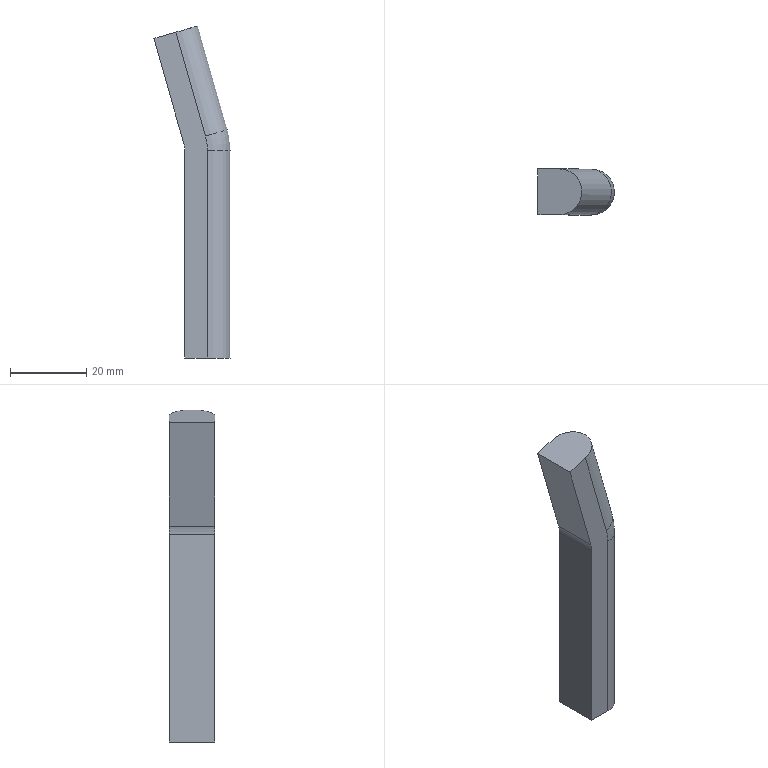Part | NX | features solid 2 | 1 solid | 10 faces | box 20.071 x 12 x 87.272 mm | volume 11133 mm3 | plane 6 | cylinder 3 | torus 1 | commonest cylinder face diameters 12 x2 16 x1
STEP:
#1=CARTESIAN_POINT('',(-548.,484.,14.523));
#2=VERTEX_POINT('',#1);
#3=CARTESIAN_POINT('',(-548.,496.,14.523));
#4=VERTEX_POINT('',#3);
#5=CARTESIAN_POINT('',(-548.,520.,14.523));
#6=DIRECTION('',(0.,1.,0.));
#7=VECTOR('',#6,1000.);
#8=LINE('',#5,#7);
#9=EDGE_CURVE('',#2,#4,#8,.T.);
#10=ORIENTED_EDGE('',*,*,#9,.T.);
#11=CARTESIAN_POINT('',(-548.,496.,-40.));
#12=VERTEX_POINT('',#11);
#13=CARTESIAN_POINT('',(-548.,496.,49.523));
#14=DIRECTION('',(0.,0.,-1.));
#15=VECTOR('',#14,1000.);
#16=LINE('',#13,#15);
#17=EDGE_CURVE('',#4,#12,#16,.T.);
#18=ORIENTED_EDGE('',*,*,#17,.T.);
#19=CARTESIAN_POINT('',(-548.,484.,-40.));
#20=VERTEX_POINT('',#19);
#21=CARTESIAN_POINT('',(-548.,463.,-40.));
#22=DIRECTION('',(0.,1.,0.));
#23=VECTOR('',#22,1000.);
#24=LINE('',#21,#23);
#25=EDGE_CURVE('',#20,#12,#24,.T.);
#26=ORIENTED_EDGE('',*,*,#25,.F.);
#27=CARTESIAN_POINT('',(-548.,484.,49.523));
#28=DIRECTION('',(0.,0.,-1.));
#29=VECTOR('',#28,1000.);
#30=LINE('',#27,#29);
#31=EDGE_CURVE('',#2,#20,#30,.T.);
#32=ORIENTED_EDGE('',*,*,#31,.F.);
#33=EDGE_LOOP('',(#10,#18,#26,#32));
#34=FACE_BOUND('',#33,.T.);
#35=CARTESIAN_POINT('',(-548.,520.,49.523));
#36=DIRECTION('',(1.,0.,0.));
#37=DIRECTION('',(0.,-1.,0.));
#38=AXIS2_PLACEMENT_3D('',#35,#36,#37);
#39=PLANE('',#38);
#40=ADVANCED_FACE('',(#34),#39,.F.);
#41=CARTESIAN_POINT('',(-542.,496.,14.523));
#42=VERTEX_POINT('',#41);
#43=CARTESIAN_POINT('',(-542.,484.,14.523));
#44=VERTEX_POINT('',#43);
#45=CARTESIAN_POINT('',(-542.,490.,14.523));
#46=DIRECTION('',(0.,0.,-1.));
#47=DIRECTION('',(1.,0.,0.));
#48=AXIS2_PLACEMENT_3D('',#45,#46,#47);
#49=CIRCLE('',#48,6.);
#50=EDGE_CURVE('',#42,#44,#49,.T.);
#51=ORIENTED_EDGE('',*,*,#50,.F.);
#52=CARTESIAN_POINT('',(-542.535,496.,18.357));
#53=VERTEX_POINT('',#52);
#54=CARTESIAN_POINT('',(-556.,496.,14.523));
#55=DIRECTION('',(0.,-1.,0.));
#56=DIRECTION('',(0.,0.,-1.));
#57=AXIS2_PLACEMENT_3D('',#54,#55,#56);
#58=CIRCLE('',#57,14.);
#59=EDGE_CURVE('',#42,#53,#58,.T.);
#60=ORIENTED_EDGE('',*,*,#59,.T.);
#61=CARTESIAN_POINT('',(-542.535,484.,18.357));
#62=VERTEX_POINT('',#61);
#63=CARTESIAN_POINT('',(-542.535,490.,18.357));
#64=DIRECTION('',(0.2738,0.,-0.9618));
#65=DIRECTION('',(0.9618,0.,0.2738));
#66=AXIS2_PLACEMENT_3D('',#63,#64,#65);
#67=CIRCLE('',#66,6.);
#68=EDGE_CURVE('',#53,#62,#67,.T.);
#69=ORIENTED_EDGE('',*,*,#68,.T.);
#70=CARTESIAN_POINT('',(-556.,484.,14.523));
#71=DIRECTION('',(0.,-1.,0.));
#72=DIRECTION('',(0.,0.,-1.));
#73=AXIS2_PLACEMENT_3D('',#70,#71,#72);
#74=CIRCLE('',#73,14.);
#75=EDGE_CURVE('',#44,#62,#74,.T.);
#76=ORIENTED_EDGE('',*,*,#75,.F.);
#77=EDGE_LOOP('',(#51,#60,#69,#76));
#78=FACE_BOUND('',#77,.T.);
#79=CARTESIAN_POINT('',(-556.,490.,14.523));
#80=DIRECTION('',(0.,1.,0.));
#81=DIRECTION('',(0.,0.,-1.));
#82=AXIS2_PLACEMENT_3D('',#79,#80,#81);
#83=TOROIDAL_SURFACE('',#82,14.,6.);
#84=ADVANCED_FACE('',(#78),#83,.T.);
#85=ORIENTED_EDGE('',*,*,#50,.T.);
#86=CARTESIAN_POINT('',(-542.,484.,-40.));
#87=VERTEX_POINT('',#86);
#88=CARTESIAN_POINT('',(-542.,484.,29.523));
#89=DIRECTION('',(0.,0.,-1.));
#90=VECTOR('',#89,1000.);
#91=LINE('',#88,#90);
#92=EDGE_CURVE('',#44,#87,#91,.T.);
#93=ORIENTED_EDGE('',*,*,#92,.T.);
#94=CARTESIAN_POINT('',(-542.,496.,-40.));
#95=VERTEX_POINT('',#94);
#96=CARTESIAN_POINT('',(-542.,490.,-40.));
#97=DIRECTION('',(0.,0.,1.));
#98=DIRECTION('',(1.,0.,0.));
#99=AXIS2_PLACEMENT_3D('',#96,#97,#98);
#100=CIRCLE('',#99,6.);
#101=EDGE_CURVE('',#95,#87,#100,.F.);
#102=ORIENTED_EDGE('',*,*,#101,.F.);
#103=CARTESIAN_POINT('',(-542.,496.,29.523));
#104=DIRECTION('',(0.,0.,-1.));
#105=VECTOR('',#104,1000.);
#106=LINE('',#103,#105);
#107=EDGE_CURVE('',#42,#95,#106,.T.);
#108=ORIENTED_EDGE('',*,*,#107,.F.);
#109=EDGE_LOOP('',(#85,#93,#102,#108));
#110=FACE_BOUND('',#109,.T.);
#111=CARTESIAN_POINT('',(-542.,490.,29.523));
#112=DIRECTION('',(0.,0.,-1.));
#113=DIRECTION('',(-1.,0.,0.));
#114=AXIS2_PLACEMENT_3D('',#111,#112,#113);
#115=CYLINDRICAL_SURFACE('',#114,6.);
#116=ADVANCED_FACE('',(#110),#115,.T.);
#117=CARTESIAN_POINT('',(-623.,484.,-40.));
#118=DIRECTION('',(-1.,0.,0.));
#119=VECTOR('',#118,1000.);
#120=LINE('',#117,#119);
#121=EDGE_CURVE('',#87,#20,#120,.T.);
#122=ORIENTED_EDGE('',*,*,#121,.T.);
#123=ORIENTED_EDGE('',*,*,#25,.T.);
#124=CARTESIAN_POINT('',(-623.,496.,-40.));
#125=DIRECTION('',(-1.,0.,0.));
#126=VECTOR('',#125,1000.);
#127=LINE('',#124,#126);
#128=EDGE_CURVE('',#95,#12,#127,.T.);
#129=ORIENTED_EDGE('',*,*,#128,.F.);
#130=ORIENTED_EDGE('',*,*,#101,.T.);
#131=EDGE_LOOP('',(#122,#123,#129,#130));
#132=FACE_BOUND('',#131,.T.);
#133=CARTESIAN_POINT('',(-623.,463.,-40.));
#134=DIRECTION('',(0.,0.,1.));
#135=DIRECTION('',(0.,1.,0.));
#136=AXIS2_PLACEMENT_3D('',#133,#134,#135);
#137=PLANE('',#136);
#138=ADVANCED_FACE('',(#132),#137,.F.);
#139=CARTESIAN_POINT('',(-550.3,484.,45.629));
#140=VERTEX_POINT('',#139);
#141=CARTESIAN_POINT('',(-542.535,484.,18.357));
#142=DIRECTION('',(-0.2738,0.,0.9618));
#143=VECTOR('',#142,1000.);
#144=LINE('',#141,#143);
#145=EDGE_CURVE('',#62,#140,#144,.T.);
#146=ORIENTED_EDGE('',*,*,#145,.T.);
#147=CARTESIAN_POINT('',(-556.071,484.,43.986));
#148=VERTEX_POINT('',#147);
#149=CARTESIAN_POINT('',(-557.81,484.,43.491));
#150=DIRECTION('',(-0.9618,0.,-0.2738));
#151=VECTOR('',#150,1000.);
#152=LINE('',#149,#151);
#153=EDGE_CURVE('',#140,#148,#152,.T.);
#154=ORIENTED_EDGE('',*,*,#153,.T.);
#155=CARTESIAN_POINT('',(-548.306,484.,16.714));
#156=VERTEX_POINT('',#155);
#157=CARTESIAN_POINT('',(-548.306,484.,16.714));
#158=DIRECTION('',(-0.2738,0.,0.9618));
#159=VECTOR('',#158,1000.);
#160=LINE('',#157,#159);
#161=EDGE_CURVE('',#156,#148,#160,.T.);
#162=ORIENTED_EDGE('',*,*,#161,.F.);
#163=CARTESIAN_POINT('',(-556.,484.,14.523));
#164=DIRECTION('',(0.,-1.,0.));
#165=DIRECTION('',(0.,0.,-1.));
#166=AXIS2_PLACEMENT_3D('',#163,#164,#165);
#167=CIRCLE('',#166,8.);
#168=EDGE_CURVE('',#2,#156,#167,.T.);
#169=ORIENTED_EDGE('',*,*,#168,.F.);
#170=ORIENTED_EDGE('',*,*,#31,.T.);
#171=ORIENTED_EDGE('',*,*,#121,.F.);
#172=ORIENTED_EDGE('',*,*,#92,.F.);
#173=ORIENTED_EDGE('',*,*,#75,.T.);
#174=EDGE_LOOP('',(#146,#154,#162,#169,#170,#171,#172,#173));
#175=FACE_BOUND('',#174,.T.);
#176=CARTESIAN_POINT('',(-640.,484.,39.523));
#177=DIRECTION('',(0.,1.,0.));
#178=DIRECTION('',(1.,0.,0.));
#179=AXIS2_PLACEMENT_3D('',#176,#177,#178);
#180=PLANE('',#179);
#181=ADVANCED_FACE('',(#175),#180,.F.);
#182=ORIENTED_EDGE('',*,*,#17,.F.);
#183=CARTESIAN_POINT('',(-548.306,496.,16.714));
#184=VERTEX_POINT('',#183);
#185=CARTESIAN_POINT('',(-556.,496.,14.523));
#186=DIRECTION('',(0.,-1.,0.));
#187=DIRECTION('',(0.,0.,-1.));
#188=AXIS2_PLACEMENT_3D('',#185,#186,#187);
#189=CIRCLE('',#188,8.);
#190=EDGE_CURVE('',#4,#184,#189,.T.);
#191=ORIENTED_EDGE('',*,*,#190,.T.);
#192=CARTESIAN_POINT('',(-556.071,496.,43.986));
#193=VERTEX_POINT('',#192);
#194=CARTESIAN_POINT('',(-548.306,496.,16.714));
#195=DIRECTION('',(-0.2738,0.,0.9618));
#196=VECTOR('',#195,1000.);
#197=LINE('',#194,#196);
#198=EDGE_CURVE('',#184,#193,#197,.T.);
#199=ORIENTED_EDGE('',*,*,#198,.T.);
#200=CARTESIAN_POINT('',(-550.3,496.,45.629));
#201=VERTEX_POINT('',#200);
#202=CARTESIAN_POINT('',(-557.81,496.,43.491));
#203=DIRECTION('',(-0.9618,0.,-0.2738));
#204=VECTOR('',#203,1000.);
#205=LINE('',#202,#204);
#206=EDGE_CURVE('',#201,#193,#205,.T.);
#207=ORIENTED_EDGE('',*,*,#206,.F.);
#208=CARTESIAN_POINT('',(-542.535,496.,18.357));
#209=DIRECTION('',(-0.2738,0.,0.9618));
#210=VECTOR('',#209,1000.);
#211=LINE('',#208,#210);
#212=EDGE_CURVE('',#53,#201,#211,.T.);
#213=ORIENTED_EDGE('',*,*,#212,.F.);
#214=ORIENTED_EDGE('',*,*,#59,.F.);
#215=ORIENTED_EDGE('',*,*,#107,.T.);
#216=ORIENTED_EDGE('',*,*,#128,.T.);
#217=EDGE_LOOP('',(#182,#191,#199,#207,#213,#214,#215,#216));
#218=FACE_BOUND('',#217,.T.);
#219=CARTESIAN_POINT('',(-640.,496.,39.523));
#220=DIRECTION('',(0.,1.,0.));
#221=DIRECTION('',(1.,0.,0.));
#222=AXIS2_PLACEMENT_3D('',#219,#220,#221);
#223=PLANE('',#222);
#224=ADVANCED_FACE('',(#218),#223,.T.);
#225=CARTESIAN_POINT('',(-550.3,490.,45.629));
#226=DIRECTION('',(-0.2738,0.,0.9618));
#227=DIRECTION('',(0.9618,0.,0.2738));
#228=AXIS2_PLACEMENT_3D('',#225,#226,#227);
#229=CIRCLE('',#228,6.);
#230=EDGE_CURVE('',#201,#140,#229,.F.);
#231=ORIENTED_EDGE('',*,*,#230,.F.);
#232=ORIENTED_EDGE('',*,*,#206,.T.);
#233=CARTESIAN_POINT('',(-556.071,520.,43.986));
#234=DIRECTION('',(0.,1.,0.));
#235=VECTOR('',#234,1000.);
#236=LINE('',#233,#235);
#237=EDGE_CURVE('',#148,#193,#236,.T.);
#238=ORIENTED_EDGE('',*,*,#237,.F.);
#239=ORIENTED_EDGE('',*,*,#153,.F.);
#240=EDGE_LOOP('',(#231,#232,#238,#239));
#241=FACE_BOUND('',#240,.T.);
#242=CARTESIAN_POINT('',(-557.81,549.75,43.491));
#243=DIRECTION('',(-0.2738,0.,0.9618));
#244=DIRECTION('',(0.9618,0.,0.2738));
#245=AXIS2_PLACEMENT_3D('',#242,#243,#244);
#246=PLANE('',#245);
#247=ADVANCED_FACE('',(#241),#246,.T.);
#248=ORIENTED_EDGE('',*,*,#212,.T.);
#249=ORIENTED_EDGE('',*,*,#230,.T.);
#250=ORIENTED_EDGE('',*,*,#145,.F.);
#251=ORIENTED_EDGE('',*,*,#68,.F.);
#252=EDGE_LOOP('',(#248,#249,#250,#251));
#253=FACE_BOUND('',#252,.T.);
#254=CARTESIAN_POINT('',(-542.535,490.,18.357));
#255=DIRECTION('',(-0.2738,0.,0.9618));
#256=DIRECTION('',(0.9618,0.,0.2738));
#257=AXIS2_PLACEMENT_3D('',#254,#255,#256);
#258=CYLINDRICAL_SURFACE('',#257,6.);
#259=ADVANCED_FACE('',(#253),#258,.T.);
#260=CARTESIAN_POINT('',(-548.306,520.,16.714));
#261=DIRECTION('',(0.,1.,0.));
#262=VECTOR('',#261,1000.);
#263=LINE('',#260,#262);
#264=EDGE_CURVE('',#156,#184,#263,.T.);
#265=ORIENTED_EDGE('',*,*,#264,.F.);
#266=ORIENTED_EDGE('',*,*,#161,.T.);
#267=ORIENTED_EDGE('',*,*,#237,.T.);
#268=ORIENTED_EDGE('',*,*,#198,.F.);
#269=EDGE_LOOP('',(#265,#266,#267,#268));
#270=FACE_BOUND('',#269,.T.);
#271=CARTESIAN_POINT('',(-548.306,520.,16.714));
#272=DIRECTION('',(-0.9618,0.,-0.2738));
#273=DIRECTION('',(-0.2738,0.,0.9618));
#274=AXIS2_PLACEMENT_3D('',#271,#272,#273);
#275=PLANE('',#274);
#276=ADVANCED_FACE('',(#270),#275,.T.);
#277=ORIENTED_EDGE('',*,*,#9,.F.);
#278=ORIENTED_EDGE('',*,*,#168,.T.);
#279=ORIENTED_EDGE('',*,*,#264,.T.);
#280=ORIENTED_EDGE('',*,*,#190,.F.);
#281=EDGE_LOOP('',(#277,#278,#279,#280));
#282=FACE_BOUND('',#281,.T.);
#283=CARTESIAN_POINT('',(-556.,535.,14.523));
#284=DIRECTION('',(0.,1.,0.));
#285=DIRECTION('',(0.,0.,-1.));
#286=AXIS2_PLACEMENT_3D('',#283,#284,#285);
#287=CYLINDRICAL_SURFACE('',#286,8.);
#288=ADVANCED_FACE('',(#282),#287,.F.);
#289=CLOSED_SHELL('',(#40,#84,#116,#138,#181,#224,#247,#259,#276,#288));
#290=MANIFOLD_SOLID_BREP('',#289);
#291=(LENGTH_UNIT()NAMED_UNIT(*)SI_UNIT(.MILLI.,.METRE.));
#292=UNCERTAINTY_MEASURE_WITH_UNIT(LENGTH_MEASURE(0.00001),#291,'','');
#293=(NAMED_UNIT(*)PLANE_ANGLE_UNIT()SI_UNIT($,.RADIAN.));
#294=(NAMED_UNIT(*)SI_UNIT($,.STERADIAN.)SOLID_ANGLE_UNIT());
#295=(GEOMETRIC_REPRESENTATION_CONTEXT(3)GLOBAL_UNCERTAINTY_ASSIGNED_CONTEXT((#292))GLOBAL_UNIT_ASSIGNED_CONTEXT((#291,#293,#294))REPRESENTATION_CONTEXT('',''));
#296=ADVANCED_BREP_SHAPE_REPRESENTATION('',(#290),#295);